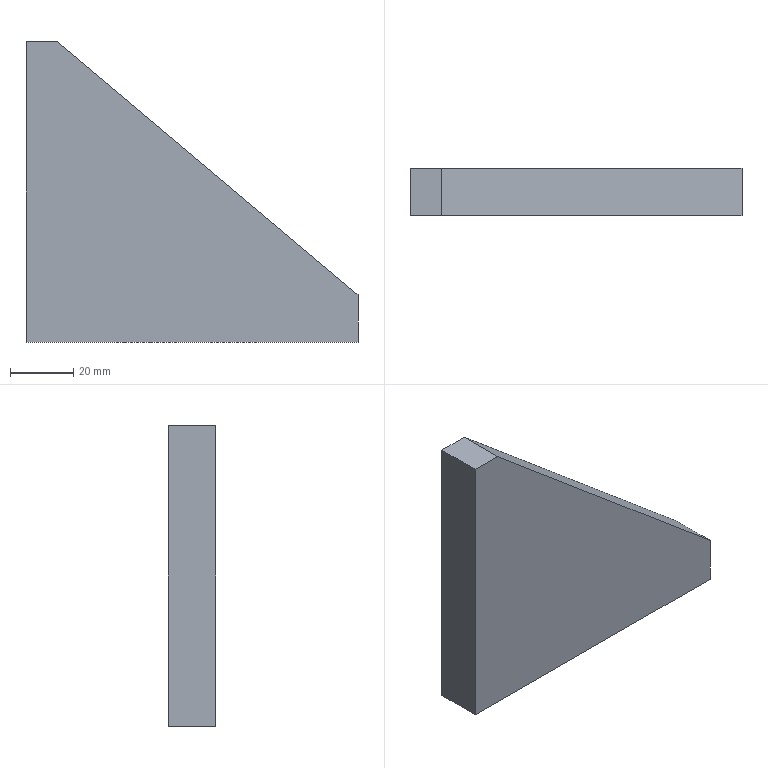Part | STEP file | Tube feed_id578_x_t | 1 solid | 7 faces | box 105 x 15 x 95 mm | volume 92625 mm3 | plane 7
STEP:
#1=CARTESIAN_POINT('',(0.,0.,0.));
#2=DIRECTION('',(0.,0.,1.));
#3=DIRECTION('',(1.,0.,0.));
#4=AXIS2_PLACEMENT_3D('',#1,#2,#3);
#5=CARTESIAN_POINT('',(511.,541.936,-204.));
#6=VERTEX_POINT('',#5);
#7=CARTESIAN_POINT('',(511.,541.936,-109.));
#8=VERTEX_POINT('',#7);
#9=CARTESIAN_POINT('',(511.,541.936,-204.));
#10=DIRECTION('',(0.,0.,1.));
#11=VECTOR('',#10,1.);
#12=LINE('',#9,#11);
#13=CARTESIAN_POINT('',(511.,571.936,-204.));
#14=DIRECTION('',(1.,0.,0.));
#15=DIRECTION('',(0.,0.,-1.));
#16=AXIS2_PLACEMENT_3D('',#13,#14,#15);
#17=PLANE('',#16);
#18=CARTESIAN_POINT('',(0.,-30.));
#19=DIRECTION('',(-1.,0.));
#20=VECTOR('',#19,1.);
#21=LINE('',#18,#20);
#22=(GEOMETRIC_REPRESENTATION_CONTEXT(2)PARAMETRIC_REPRESENTATION_CONTEXT()REPRESENTATION_CONTEXT('',''));
#23=DEFINITIONAL_REPRESENTATION('',(#21),#22);
#24=PCURVE('',#17,#23);
#25=CARTESIAN_POINT('',(503.5,541.936,-156.5));
#26=DIRECTION('',(0.,1.,0.));
#27=DIRECTION('',(0.,0.,1.));
#28=AXIS2_PLACEMENT_3D('',#25,#26,#27);
#29=PLANE('',#28);
#30=CARTESIAN_POINT('',(-47.5,7.5));
#31=DIRECTION('',(1.,0.));
#32=VECTOR('',#31,1.);
#33=LINE('',#30,#32);
#34=(GEOMETRIC_REPRESENTATION_CONTEXT(2)PARAMETRIC_REPRESENTATION_CONTEXT()REPRESENTATION_CONTEXT('',''));
#35=DEFINITIONAL_REPRESENTATION('',(#33),#34);
#36=PCURVE('',#29,#35);
#37=SURFACE_CURVE('',#12,(#24,#36),.PCURVE_S1.);
#38=EDGE_CURVE('',#6,#8,#37,.T.);
#39=ORIENTED_EDGE('',*,*,#38,.F.);
#40=CARTESIAN_POINT('',(511.,526.936,-204.));
#41=VERTEX_POINT('',#40);
#42=CARTESIAN_POINT('',(511.,571.936,-204.));
#43=DIRECTION('',(0.,-1.,0.));
#44=VECTOR('',#43,1.);
#45=LINE('',#42,#44);
#46=CARTESIAN_POINT('',(0.,0.));
#47=DIRECTION('',(0.,-1.));
#48=VECTOR('',#47,1.);
#49=LINE('',#46,#48);
#50=(GEOMETRIC_REPRESENTATION_CONTEXT(2)PARAMETRIC_REPRESENTATION_CONTEXT()REPRESENTATION_CONTEXT('',''));
#51=DEFINITIONAL_REPRESENTATION('',(#49),#50);
#52=PCURVE('',#17,#51);
#53=CARTESIAN_POINT('',(616.,571.936,-204.));
#54=DIRECTION('',(0.,0.,1.));
#55=DIRECTION('',(1.,0.,0.));
#56=AXIS2_PLACEMENT_3D('',#53,#54,#55);
#57=PLANE('',#56);
#58=CARTESIAN_POINT('',(-105.,0.));
#59=DIRECTION('',(0.,-1.));
#60=VECTOR('',#59,1.);
#61=LINE('',#58,#60);
#62=(GEOMETRIC_REPRESENTATION_CONTEXT(2)PARAMETRIC_REPRESENTATION_CONTEXT()REPRESENTATION_CONTEXT('',''));
#63=DEFINITIONAL_REPRESENTATION('',(#61),#62);
#64=PCURVE('',#57,#63);
#65=SURFACE_CURVE('',#45,(#52,#64),.PCURVE_S1.);
#66=EDGE_CURVE('',#6,#41,#65,.T.);
#67=ORIENTED_EDGE('',*,*,#66,.T.);
#68=CARTESIAN_POINT('',(511.,526.936,-109.));
#69=VERTEX_POINT('',#68);
#70=CARTESIAN_POINT('',(511.,526.936,-204.));
#71=DIRECTION('',(0.,0.,1.));
#72=VECTOR('',#71,1.);
#73=LINE('',#70,#72);
#74=CARTESIAN_POINT('',(0.,-45.));
#75=DIRECTION('',(-1.,0.));
#76=VECTOR('',#75,1.);
#77=LINE('',#74,#76);
#78=(GEOMETRIC_REPRESENTATION_CONTEXT(2)PARAMETRIC_REPRESENTATION_CONTEXT()REPRESENTATION_CONTEXT('',''));
#79=DEFINITIONAL_REPRESENTATION('',(#77),#78);
#80=PCURVE('',#17,#79);
#81=CARTESIAN_POINT('',(0.,526.936,0.));
#82=DIRECTION('',(0.,1.,0.));
#83=DIRECTION('',(0.,0.,1.));
#84=AXIS2_PLACEMENT_3D('',#81,#82,#83);
#85=PLANE('',#84);
#86=CARTESIAN_POINT('',(-204.,511.));
#87=DIRECTION('',(1.,0.));
#88=VECTOR('',#87,1.);
#89=LINE('',#86,#88);
#90=(GEOMETRIC_REPRESENTATION_CONTEXT(2)PARAMETRIC_REPRESENTATION_CONTEXT()REPRESENTATION_CONTEXT('',''));
#91=DEFINITIONAL_REPRESENTATION('',(#89),#90);
#92=PCURVE('',#85,#91);
#93=SURFACE_CURVE('',#73,(#80,#92),.PCURVE_S1.);
#94=EDGE_CURVE('',#41,#69,#93,.T.);
#95=ORIENTED_EDGE('',*,*,#94,.T.);
#96=CARTESIAN_POINT('',(511.,571.936,-109.));
#97=DIRECTION('',(0.,-1.,0.));
#98=VECTOR('',#97,1.);
#99=LINE('',#96,#98);
#100=CARTESIAN_POINT('',(-95.,0.));
#101=DIRECTION('',(0.,-1.));
#102=VECTOR('',#101,1.);
#103=LINE('',#100,#102);
#104=(GEOMETRIC_REPRESENTATION_CONTEXT(2)PARAMETRIC_REPRESENTATION_CONTEXT()REPRESENTATION_CONTEXT('',''));
#105=DEFINITIONAL_REPRESENTATION('',(#103),#104);
#106=PCURVE('',#17,#105);
#107=CARTESIAN_POINT('',(511.,571.936,-109.));
#108=DIRECTION('',(0.,0.,-1.));
#109=DIRECTION('',(-1.,0.,0.));
#110=AXIS2_PLACEMENT_3D('',#107,#108,#109);
#111=PLANE('',#110);
#112=CARTESIAN_POINT('',(0.,0.));
#113=DIRECTION('',(0.,-1.));
#114=VECTOR('',#113,1.);
#115=LINE('',#112,#114);
#116=(GEOMETRIC_REPRESENTATION_CONTEXT(2)PARAMETRIC_REPRESENTATION_CONTEXT()REPRESENTATION_CONTEXT('',''));
#117=DEFINITIONAL_REPRESENTATION('',(#115),#116);
#118=PCURVE('',#111,#117);
#119=SURFACE_CURVE('',#99,(#106,#118),.PCURVE_S1.);
#120=EDGE_CURVE('',#8,#69,#119,.T.);
#121=ORIENTED_EDGE('',*,*,#120,.F.);
#122=EDGE_LOOP('',(#39,#67,#95,#121));
#123=FACE_BOUND('',#122,.T.);
#124=ADVANCED_FACE('',(#123),#17,.F.);
#125=CARTESIAN_POINT('',(521.,541.936,-109.));
#126=VERTEX_POINT('',#125);
#127=CARTESIAN_POINT('',(511.,541.936,-109.));
#128=DIRECTION('',(1.,0.,0.));
#129=VECTOR('',#128,1.);
#130=LINE('',#127,#129);
#131=CARTESIAN_POINT('',(0.,-30.));
#132=DIRECTION('',(-1.,0.));
#133=VECTOR('',#132,1.);
#134=LINE('',#131,#133);
#135=(GEOMETRIC_REPRESENTATION_CONTEXT(2)PARAMETRIC_REPRESENTATION_CONTEXT()REPRESENTATION_CONTEXT('',''));
#136=DEFINITIONAL_REPRESENTATION('',(#134),#135);
#137=PCURVE('',#111,#136);
#138=CARTESIAN_POINT('',(47.5,7.5));
#139=DIRECTION('',(0.,1.));
#140=VECTOR('',#139,1.);
#141=LINE('',#138,#140);
#142=(GEOMETRIC_REPRESENTATION_CONTEXT(2)PARAMETRIC_REPRESENTATION_CONTEXT()REPRESENTATION_CONTEXT('',''));
#143=DEFINITIONAL_REPRESENTATION('',(#141),#142);
#144=PCURVE('',#29,#143);
#145=SURFACE_CURVE('',#130,(#137,#144),.PCURVE_S1.);
#146=EDGE_CURVE('',#8,#126,#145,.T.);
#147=ORIENTED_EDGE('',*,*,#146,.F.);
#148=ORIENTED_EDGE('',*,*,#120,.T.);
#149=CARTESIAN_POINT('',(521.,526.936,-109.));
#150=VERTEX_POINT('',#149);
#151=CARTESIAN_POINT('',(511.,526.936,-109.));
#152=DIRECTION('',(1.,0.,0.));
#153=VECTOR('',#152,1.);
#154=LINE('',#151,#153);
#155=CARTESIAN_POINT('',(0.,-45.));
#156=DIRECTION('',(-1.,0.));
#157=VECTOR('',#156,1.);
#158=LINE('',#155,#157);
#159=(GEOMETRIC_REPRESENTATION_CONTEXT(2)PARAMETRIC_REPRESENTATION_CONTEXT()REPRESENTATION_CONTEXT('',''));
#160=DEFINITIONAL_REPRESENTATION('',(#158),#159);
#161=PCURVE('',#111,#160);
#162=CARTESIAN_POINT('',(-109.,511.));
#163=DIRECTION('',(0.,1.));
#164=VECTOR('',#163,1.);
#165=LINE('',#162,#164);
#166=(GEOMETRIC_REPRESENTATION_CONTEXT(2)PARAMETRIC_REPRESENTATION_CONTEXT()REPRESENTATION_CONTEXT('',''));
#167=DEFINITIONAL_REPRESENTATION('',(#165),#166);
#168=PCURVE('',#85,#167);
#169=SURFACE_CURVE('',#154,(#161,#168),.PCURVE_S1.);
#170=EDGE_CURVE('',#69,#150,#169,.T.);
#171=ORIENTED_EDGE('',*,*,#170,.T.);
#172=CARTESIAN_POINT('',(521.,571.936,-109.));
#173=DIRECTION('',(0.,-1.,0.));
#174=VECTOR('',#173,1.);
#175=LINE('',#172,#174);
#176=CARTESIAN_POINT('',(-10.,0.));
#177=DIRECTION('',(0.,-1.));
#178=VECTOR('',#177,1.);
#179=LINE('',#176,#178);
#180=(GEOMETRIC_REPRESENTATION_CONTEXT(2)PARAMETRIC_REPRESENTATION_CONTEXT()REPRESENTATION_CONTEXT('',''));
#181=DEFINITIONAL_REPRESENTATION('',(#179),#180);
#182=PCURVE('',#111,#181);
#183=CARTESIAN_POINT('',(521.,571.936,-109.));
#184=DIRECTION('',(-0.6441,0.,-0.7649));
#185=DIRECTION('',(-0.7649,0.,0.6441));
#186=AXIS2_PLACEMENT_3D('',#183,#184,#185);
#187=PLANE('',#186);
#188=CARTESIAN_POINT('',(0.,0.));
#189=DIRECTION('',(0.,-1.));
#190=VECTOR('',#189,1.);
#191=LINE('',#188,#190);
#192=(GEOMETRIC_REPRESENTATION_CONTEXT(2)PARAMETRIC_REPRESENTATION_CONTEXT()REPRESENTATION_CONTEXT('',''));
#193=DEFINITIONAL_REPRESENTATION('',(#191),#192);
#194=PCURVE('',#187,#193);
#195=SURFACE_CURVE('',#175,(#182,#194),.PCURVE_S1.);
#196=EDGE_CURVE('',#126,#150,#195,.T.);
#197=ORIENTED_EDGE('',*,*,#196,.F.);
#198=EDGE_LOOP('',(#147,#148,#171,#197));
#199=FACE_BOUND('',#198,.T.);
#200=ADVANCED_FACE('',(#199),#111,.F.);
#201=CARTESIAN_POINT('',(616.,541.936,-189.));
#202=VERTEX_POINT('',#201);
#203=CARTESIAN_POINT('',(521.,541.936,-109.));
#204=DIRECTION('',(0.7649,0.,-0.6441));
#205=VECTOR('',#204,1.);
#206=LINE('',#203,#205);
#207=CARTESIAN_POINT('',(0.,-30.));
#208=DIRECTION('',(-1.,0.));
#209=VECTOR('',#208,1.);
#210=LINE('',#207,#209);
#211=(GEOMETRIC_REPRESENTATION_CONTEXT(2)PARAMETRIC_REPRESENTATION_CONTEXT()REPRESENTATION_CONTEXT('',''));
#212=DEFINITIONAL_REPRESENTATION('',(#210),#211);
#213=PCURVE('',#187,#212);
#214=CARTESIAN_POINT('',(47.5,17.5));
#215=DIRECTION('',(-0.6441,0.7649));
#216=VECTOR('',#215,1.);
#217=LINE('',#214,#216);
#218=(GEOMETRIC_REPRESENTATION_CONTEXT(2)PARAMETRIC_REPRESENTATION_CONTEXT()REPRESENTATION_CONTEXT('',''));
#219=DEFINITIONAL_REPRESENTATION('',(#217),#218);
#220=PCURVE('',#29,#219);
#221=SURFACE_CURVE('',#206,(#213,#220),.PCURVE_S1.);
#222=EDGE_CURVE('',#126,#202,#221,.T.);
#223=ORIENTED_EDGE('',*,*,#222,.F.);
#224=ORIENTED_EDGE('',*,*,#196,.T.);
#225=CARTESIAN_POINT('',(616.,526.936,-189.));
#226=VERTEX_POINT('',#225);
#227=CARTESIAN_POINT('',(521.,526.936,-109.));
#228=DIRECTION('',(0.7649,0.,-0.6441));
#229=VECTOR('',#228,1.);
#230=LINE('',#227,#229);
#231=CARTESIAN_POINT('',(0.,-45.));
#232=DIRECTION('',(-1.,0.));
#233=VECTOR('',#232,1.);
#234=LINE('',#231,#233);
#235=(GEOMETRIC_REPRESENTATION_CONTEXT(2)PARAMETRIC_REPRESENTATION_CONTEXT()REPRESENTATION_CONTEXT('',''));
#236=DEFINITIONAL_REPRESENTATION('',(#234),#235);
#237=PCURVE('',#187,#236);
#238=CARTESIAN_POINT('',(-109.,521.));
#239=DIRECTION('',(-0.6441,0.7649));
#240=VECTOR('',#239,1.);
#241=LINE('',#238,#240);
#242=(GEOMETRIC_REPRESENTATION_CONTEXT(2)PARAMETRIC_REPRESENTATION_CONTEXT()REPRESENTATION_CONTEXT('',''));
#243=DEFINITIONAL_REPRESENTATION('',(#241),#242);
#244=PCURVE('',#85,#243);
#245=SURFACE_CURVE('',#230,(#237,#244),.PCURVE_S1.);
#246=EDGE_CURVE('',#150,#226,#245,.T.);
#247=ORIENTED_EDGE('',*,*,#246,.T.);
#248=CARTESIAN_POINT('',(616.,571.936,-189.));
#249=DIRECTION('',(0.,-1.,0.));
#250=VECTOR('',#249,1.);
#251=LINE('',#248,#250);
#252=CARTESIAN_POINT('',(-124.197,0.));
#253=DIRECTION('',(0.,-1.));
#254=VECTOR('',#253,1.);
#255=LINE('',#252,#254);
#256=(GEOMETRIC_REPRESENTATION_CONTEXT(2)PARAMETRIC_REPRESENTATION_CONTEXT()REPRESENTATION_CONTEXT('',''));
#257=DEFINITIONAL_REPRESENTATION('',(#255),#256);
#258=PCURVE('',#187,#257);
#259=CARTESIAN_POINT('',(616.,571.936,-189.));
#260=DIRECTION('',(-1.,0.,0.));
#261=DIRECTION('',(0.,0.,1.));
#262=AXIS2_PLACEMENT_3D('',#259,#260,#261);
#263=PLANE('',#262);
#264=CARTESIAN_POINT('',(0.,0.));
#265=DIRECTION('',(0.,-1.));
#266=VECTOR('',#265,1.);
#267=LINE('',#264,#266);
#268=(GEOMETRIC_REPRESENTATION_CONTEXT(2)PARAMETRIC_REPRESENTATION_CONTEXT()REPRESENTATION_CONTEXT('',''));
#269=DEFINITIONAL_REPRESENTATION('',(#267),#268);
#270=PCURVE('',#263,#269);
#271=SURFACE_CURVE('',#251,(#258,#270),.PCURVE_S1.);
#272=EDGE_CURVE('',#202,#226,#271,.T.);
#273=ORIENTED_EDGE('',*,*,#272,.F.);
#274=EDGE_LOOP('',(#223,#224,#247,#273));
#275=FACE_BOUND('',#274,.T.);
#276=ADVANCED_FACE('',(#275),#187,.F.);
#277=CARTESIAN_POINT('',(616.,541.936,-204.));
#278=VERTEX_POINT('',#277);
#279=CARTESIAN_POINT('',(616.,541.936,-189.));
#280=DIRECTION('',(0.,0.,-1.));
#281=VECTOR('',#280,1.);
#282=LINE('',#279,#281);
#283=CARTESIAN_POINT('',(0.,-30.));
#284=DIRECTION('',(-1.,0.));
#285=VECTOR('',#284,1.);
#286=LINE('',#283,#285);
#287=(GEOMETRIC_REPRESENTATION_CONTEXT(2)PARAMETRIC_REPRESENTATION_CONTEXT()REPRESENTATION_CONTEXT('',''));
#288=DEFINITIONAL_REPRESENTATION('',(#286),#287);
#289=PCURVE('',#263,#288);
#290=CARTESIAN_POINT('',(-32.5,112.5));
#291=DIRECTION('',(-1.,0.));
#292=VECTOR('',#291,1.);
#293=LINE('',#290,#292);
#294=(GEOMETRIC_REPRESENTATION_CONTEXT(2)PARAMETRIC_REPRESENTATION_CONTEXT()REPRESENTATION_CONTEXT('',''));
#295=DEFINITIONAL_REPRESENTATION('',(#293),#294);
#296=PCURVE('',#29,#295);
#297=SURFACE_CURVE('',#282,(#289,#296),.PCURVE_S1.);
#298=EDGE_CURVE('',#202,#278,#297,.T.);
#299=ORIENTED_EDGE('',*,*,#298,.F.);
#300=ORIENTED_EDGE('',*,*,#272,.T.);
#301=CARTESIAN_POINT('',(616.,526.936,-204.));
#302=VERTEX_POINT('',#301);
#303=CARTESIAN_POINT('',(616.,526.936,-189.));
#304=DIRECTION('',(0.,0.,-1.));
#305=VECTOR('',#304,1.);
#306=LINE('',#303,#305);
#307=CARTESIAN_POINT('',(0.,-45.));
#308=DIRECTION('',(-1.,0.));
#309=VECTOR('',#308,1.);
#310=LINE('',#307,#309);
#311=(GEOMETRIC_REPRESENTATION_CONTEXT(2)PARAMETRIC_REPRESENTATION_CONTEXT()REPRESENTATION_CONTEXT('',''));
#312=DEFINITIONAL_REPRESENTATION('',(#310),#311);
#313=PCURVE('',#263,#312);
#314=CARTESIAN_POINT('',(-189.,616.));
#315=DIRECTION('',(-1.,0.));
#316=VECTOR('',#315,1.);
#317=LINE('',#314,#316);
#318=(GEOMETRIC_REPRESENTATION_CONTEXT(2)PARAMETRIC_REPRESENTATION_CONTEXT()REPRESENTATION_CONTEXT('',''));
#319=DEFINITIONAL_REPRESENTATION('',(#317),#318);
#320=PCURVE('',#85,#319);
#321=SURFACE_CURVE('',#306,(#313,#320),.PCURVE_S1.);
#322=EDGE_CURVE('',#226,#302,#321,.T.);
#323=ORIENTED_EDGE('',*,*,#322,.T.);
#324=CARTESIAN_POINT('',(616.,571.936,-204.));
#325=DIRECTION('',(0.,-1.,0.));
#326=VECTOR('',#325,1.);
#327=LINE('',#324,#326);
#328=CARTESIAN_POINT('',(-15.,0.));
#329=DIRECTION('',(0.,-1.));
#330=VECTOR('',#329,1.);
#331=LINE('',#328,#330);
#332=(GEOMETRIC_REPRESENTATION_CONTEXT(2)PARAMETRIC_REPRESENTATION_CONTEXT()REPRESENTATION_CONTEXT('',''));
#333=DEFINITIONAL_REPRESENTATION('',(#331),#332);
#334=PCURVE('',#263,#333);
#335=CARTESIAN_POINT('',(0.,0.));
#336=DIRECTION('',(0.,-1.));
#337=VECTOR('',#336,1.);
#338=LINE('',#335,#337);
#339=(GEOMETRIC_REPRESENTATION_CONTEXT(2)PARAMETRIC_REPRESENTATION_CONTEXT()REPRESENTATION_CONTEXT('',''));
#340=DEFINITIONAL_REPRESENTATION('',(#338),#339);
#341=PCURVE('',#57,#340);
#342=SURFACE_CURVE('',#327,(#334,#341),.PCURVE_S1.);
#343=EDGE_CURVE('',#278,#302,#342,.T.);
#344=ORIENTED_EDGE('',*,*,#343,.F.);
#345=EDGE_LOOP('',(#299,#300,#323,#344));
#346=FACE_BOUND('',#345,.T.);
#347=ADVANCED_FACE('',(#346),#263,.F.);
#348=CARTESIAN_POINT('',(616.,541.936,-204.));
#349=DIRECTION('',(-1.,0.,0.));
#350=VECTOR('',#349,1.);
#351=LINE('',#348,#350);
#352=CARTESIAN_POINT('',(0.,-30.));
#353=DIRECTION('',(-1.,0.));
#354=VECTOR('',#353,1.);
#355=LINE('',#352,#354);
#356=(GEOMETRIC_REPRESENTATION_CONTEXT(2)PARAMETRIC_REPRESENTATION_CONTEXT()REPRESENTATION_CONTEXT('',''));
#357=DEFINITIONAL_REPRESENTATION('',(#355),#356);
#358=PCURVE('',#57,#357);
#359=CARTESIAN_POINT('',(-47.5,112.5));
#360=DIRECTION('',(0.,-1.));
#361=VECTOR('',#360,1.);
#362=LINE('',#359,#361);
#363=(GEOMETRIC_REPRESENTATION_CONTEXT(2)PARAMETRIC_REPRESENTATION_CONTEXT()REPRESENTATION_CONTEXT('',''));
#364=DEFINITIONAL_REPRESENTATION('',(#362),#363);
#365=PCURVE('',#29,#364);
#366=SURFACE_CURVE('',#351,(#358,#365),.PCURVE_S1.);
#367=EDGE_CURVE('',#278,#6,#366,.T.);
#368=ORIENTED_EDGE('',*,*,#367,.F.);
#369=ORIENTED_EDGE('',*,*,#343,.T.);
#370=CARTESIAN_POINT('',(616.,526.936,-204.));
#371=DIRECTION('',(-1.,0.,0.));
#372=VECTOR('',#371,1.);
#373=LINE('',#370,#372);
#374=CARTESIAN_POINT('',(0.,-45.));
#375=DIRECTION('',(-1.,0.));
#376=VECTOR('',#375,1.);
#377=LINE('',#374,#376);
#378=(GEOMETRIC_REPRESENTATION_CONTEXT(2)PARAMETRIC_REPRESENTATION_CONTEXT()REPRESENTATION_CONTEXT('',''));
#379=DEFINITIONAL_REPRESENTATION('',(#377),#378);
#380=PCURVE('',#57,#379);
#381=CARTESIAN_POINT('',(-204.,616.));
#382=DIRECTION('',(0.,-1.));
#383=VECTOR('',#382,1.);
#384=LINE('',#381,#383);
#385=(GEOMETRIC_REPRESENTATION_CONTEXT(2)PARAMETRIC_REPRESENTATION_CONTEXT()REPRESENTATION_CONTEXT('',''));
#386=DEFINITIONAL_REPRESENTATION('',(#384),#385);
#387=PCURVE('',#85,#386);
#388=SURFACE_CURVE('',#373,(#380,#387),.PCURVE_S1.);
#389=EDGE_CURVE('',#302,#41,#388,.T.);
#390=ORIENTED_EDGE('',*,*,#389,.T.);
#391=ORIENTED_EDGE('',*,*,#66,.F.);
#392=EDGE_LOOP('',(#368,#369,#390,#391));
#393=FACE_BOUND('',#392,.T.);
#394=ADVANCED_FACE('',(#393),#57,.F.);
#395=ORIENTED_EDGE('',*,*,#94,.F.);
#396=ORIENTED_EDGE('',*,*,#389,.F.);
#397=ORIENTED_EDGE('',*,*,#322,.F.);
#398=ORIENTED_EDGE('',*,*,#246,.F.);
#399=ORIENTED_EDGE('',*,*,#170,.F.);
#400=EDGE_LOOP('',(#395,#396,#397,#398,#399));
#401=FACE_BOUND('',#400,.T.);
#402=ADVANCED_FACE('',(#401),#85,.F.);
#403=ORIENTED_EDGE('',*,*,#367,.T.);
#404=ORIENTED_EDGE('',*,*,#38,.T.);
#405=ORIENTED_EDGE('',*,*,#146,.T.);
#406=ORIENTED_EDGE('',*,*,#222,.T.);
#407=ORIENTED_EDGE('',*,*,#298,.T.);
#408=EDGE_LOOP('',(#403,#404,#405,#406,#407));
#409=FACE_BOUND('',#408,.T.);
#410=ADVANCED_FACE('',(#409),#29,.T.);
#411=CLOSED_SHELL('',(#124,#200,#276,#347,#394,#402,#410));
#412=MANIFOLD_SOLID_BREP('',#411);
#413=(LENGTH_UNIT()NAMED_UNIT(*)SI_UNIT(.MILLI.,.METRE.));
#414=UNCERTAINTY_MEASURE_WITH_UNIT(LENGTH_MEASURE(0.0000001),#413,'','');
#415=(NAMED_UNIT(*)PLANE_ANGLE_UNIT()SI_UNIT($,.RADIAN.));
#416=(NAMED_UNIT(*)SI_UNIT($,.STERADIAN.)SOLID_ANGLE_UNIT());
#417=(GEOMETRIC_REPRESENTATION_CONTEXT(3)GLOBAL_UNCERTAINTY_ASSIGNED_CONTEXT((#414))GLOBAL_UNIT_ASSIGNED_CONTEXT((#413,#415,#416))REPRESENTATION_CONTEXT('',''));
#418=ADVANCED_BREP_SHAPE_REPRESENTATION('',(#4,#412),#417);